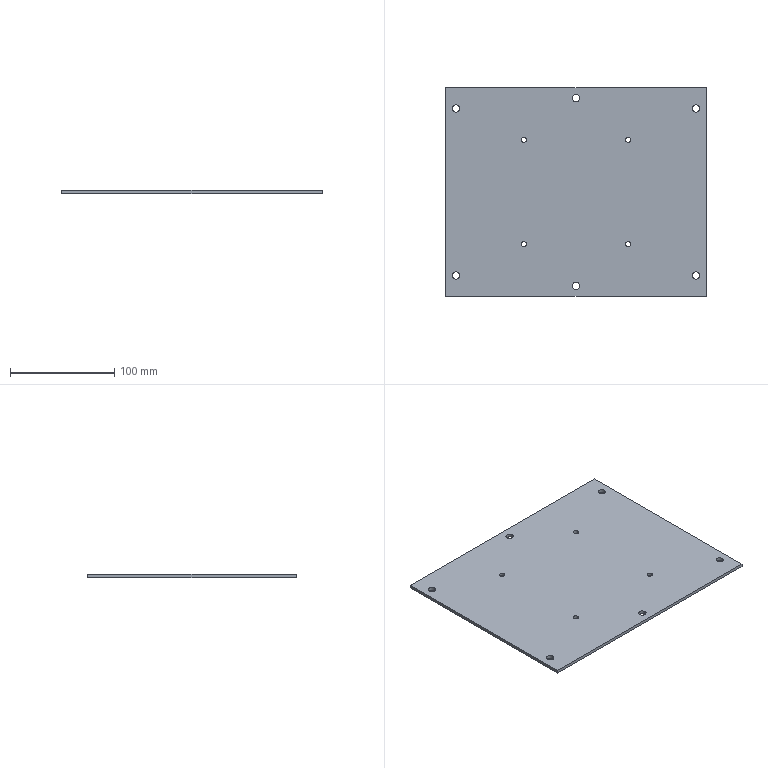Part | SolidWorks | features Cut 2, FlatPattern 1, HoleWzd 1, SMBaseFlange 1, SheetMetal 1 | 1 solid | 26 faces | box 250 x 200 x 3 mm | volume 149072 mm3 | cylinder 20 | plane 6 | commonest cylinder face diameters 7 x12 5 x8
STEP:
#1=CARTESIAN_POINT('',(52.5,50.,0.));
#2=VERTEX_POINT('',#1);
#3=CARTESIAN_POINT('',(47.5,50.,0.));
#4=VERTEX_POINT('',#3);
#5=CARTESIAN_POINT('',(50.,50.,0.));
#6=DIRECTION('',(0.,0.,-1.));
#7=DIRECTION('',(-1.,0.,0.));
#8=AXIS2_PLACEMENT_3D('',#5,#6,#7);
#9=CIRCLE('',#8,2.5);
#10=EDGE_CURVE('',#2,#4,#9,.T.);
#11=ORIENTED_EDGE('',*,*,#10,.F.);
#12=CARTESIAN_POINT('',(52.5,50.,-3.));
#13=VERTEX_POINT('',#12);
#14=CARTESIAN_POINT('',(52.5,50.,-3.));
#15=DIRECTION('',(0.,0.,-1.));
#16=VECTOR('',#15,1000.);
#17=LINE('',#14,#16);
#18=EDGE_CURVE('',#2,#13,#17,.T.);
#19=ORIENTED_EDGE('',*,*,#18,.T.);
#20=CARTESIAN_POINT('',(47.5,50.,-3.));
#21=VERTEX_POINT('',#20);
#22=CARTESIAN_POINT('',(50.,50.,-3.));
#23=DIRECTION('',(0.,0.,-1.));
#24=DIRECTION('',(-1.,0.,0.));
#25=AXIS2_PLACEMENT_3D('',#22,#23,#24);
#26=CIRCLE('',#25,2.5);
#27=EDGE_CURVE('',#13,#21,#26,.T.);
#28=ORIENTED_EDGE('',*,*,#27,.T.);
#29=CARTESIAN_POINT('',(47.5,50.,-3.));
#30=DIRECTION('',(0.,0.,-1.));
#31=VECTOR('',#30,1000.);
#32=LINE('',#29,#31);
#33=EDGE_CURVE('',#4,#21,#32,.T.);
#34=ORIENTED_EDGE('',*,*,#33,.F.);
#35=EDGE_LOOP('',(#11,#19,#28,#34));
#36=FACE_OUTER_BOUND('',#35,.T.);
#37=CARTESIAN_POINT('',(50.,50.,-3.));
#38=DIRECTION('',(0.,0.,-1.));
#39=DIRECTION('',(-1.,0.,0.));
#40=AXIS2_PLACEMENT_3D('',#37,#38,#39);
#41=CYLINDRICAL_SURFACE('',#40,2.5);
#42=ADVANCED_FACE('',(#36),#41,.F.);
#43=CARTESIAN_POINT('',(-47.5,50.,0.));
#44=VERTEX_POINT('',#43);
#45=CARTESIAN_POINT('',(-52.5,50.,0.));
#46=VERTEX_POINT('',#45);
#47=CARTESIAN_POINT('',(-50.,50.,0.));
#48=DIRECTION('',(0.,0.,-1.));
#49=DIRECTION('',(-1.,0.,0.));
#50=AXIS2_PLACEMENT_3D('',#47,#48,#49);
#51=CIRCLE('',#50,2.5);
#52=EDGE_CURVE('',#44,#46,#51,.T.);
#53=ORIENTED_EDGE('',*,*,#52,.F.);
#54=CARTESIAN_POINT('',(-47.5,50.,-3.));
#55=VERTEX_POINT('',#54);
#56=CARTESIAN_POINT('',(-47.5,50.,-3.));
#57=DIRECTION('',(0.,0.,-1.));
#58=VECTOR('',#57,1000.);
#59=LINE('',#56,#58);
#60=EDGE_CURVE('',#44,#55,#59,.T.);
#61=ORIENTED_EDGE('',*,*,#60,.T.);
#62=CARTESIAN_POINT('',(-52.5,50.,-3.));
#63=VERTEX_POINT('',#62);
#64=CARTESIAN_POINT('',(-50.,50.,-3.));
#65=DIRECTION('',(0.,0.,-1.));
#66=DIRECTION('',(-1.,0.,0.));
#67=AXIS2_PLACEMENT_3D('',#64,#65,#66);
#68=CIRCLE('',#67,2.5);
#69=EDGE_CURVE('',#55,#63,#68,.T.);
#70=ORIENTED_EDGE('',*,*,#69,.T.);
#71=CARTESIAN_POINT('',(-52.5,50.,-3.));
#72=DIRECTION('',(0.,0.,-1.));
#73=VECTOR('',#72,1000.);
#74=LINE('',#71,#73);
#75=EDGE_CURVE('',#46,#63,#74,.T.);
#76=ORIENTED_EDGE('',*,*,#75,.F.);
#77=EDGE_LOOP('',(#53,#61,#70,#76));
#78=FACE_OUTER_BOUND('',#77,.T.);
#79=CARTESIAN_POINT('',(-50.,50.,-3.));
#80=DIRECTION('',(0.,0.,-1.));
#81=DIRECTION('',(-1.,0.,0.));
#82=AXIS2_PLACEMENT_3D('',#79,#80,#81);
#83=CYLINDRICAL_SURFACE('',#82,2.5);
#84=ADVANCED_FACE('',(#78),#83,.F.);
#85=CARTESIAN_POINT('',(-47.5,-50.,0.));
#86=VERTEX_POINT('',#85);
#87=CARTESIAN_POINT('',(-52.5,-50.,0.));
#88=VERTEX_POINT('',#87);
#89=CARTESIAN_POINT('',(-50.,-50.,0.));
#90=DIRECTION('',(0.,0.,-1.));
#91=DIRECTION('',(-1.,0.,0.));
#92=AXIS2_PLACEMENT_3D('',#89,#90,#91);
#93=CIRCLE('',#92,2.5);
#94=EDGE_CURVE('',#86,#88,#93,.T.);
#95=ORIENTED_EDGE('',*,*,#94,.F.);
#96=CARTESIAN_POINT('',(-47.5,-50.,-3.));
#97=VERTEX_POINT('',#96);
#98=CARTESIAN_POINT('',(-47.5,-50.,-3.));
#99=DIRECTION('',(0.,0.,-1.));
#100=VECTOR('',#99,1000.);
#101=LINE('',#98,#100);
#102=EDGE_CURVE('',#86,#97,#101,.T.);
#103=ORIENTED_EDGE('',*,*,#102,.T.);
#104=CARTESIAN_POINT('',(-52.5,-50.,-3.));
#105=VERTEX_POINT('',#104);
#106=CARTESIAN_POINT('',(-50.,-50.,-3.));
#107=DIRECTION('',(0.,0.,-1.));
#108=DIRECTION('',(-1.,0.,0.));
#109=AXIS2_PLACEMENT_3D('',#106,#107,#108);
#110=CIRCLE('',#109,2.5);
#111=EDGE_CURVE('',#97,#105,#110,.T.);
#112=ORIENTED_EDGE('',*,*,#111,.T.);
#113=CARTESIAN_POINT('',(-52.5,-50.,-3.));
#114=DIRECTION('',(0.,0.,-1.));
#115=VECTOR('',#114,1000.);
#116=LINE('',#113,#115);
#117=EDGE_CURVE('',#88,#105,#116,.T.);
#118=ORIENTED_EDGE('',*,*,#117,.F.);
#119=EDGE_LOOP('',(#95,#103,#112,#118));
#120=FACE_OUTER_BOUND('',#119,.T.);
#121=CARTESIAN_POINT('',(-50.,-50.,-3.));
#122=DIRECTION('',(0.,0.,-1.));
#123=DIRECTION('',(-1.,0.,0.));
#124=AXIS2_PLACEMENT_3D('',#121,#122,#123);
#125=CYLINDRICAL_SURFACE('',#124,2.5);
#126=ADVANCED_FACE('',(#120),#125,.F.);
#127=CARTESIAN_POINT('',(52.5,-50.,0.));
#128=VERTEX_POINT('',#127);
#129=CARTESIAN_POINT('',(47.5,-50.,0.));
#130=VERTEX_POINT('',#129);
#131=CARTESIAN_POINT('',(50.,-50.,0.));
#132=DIRECTION('',(0.,0.,-1.));
#133=DIRECTION('',(-1.,0.,0.));
#134=AXIS2_PLACEMENT_3D('',#131,#132,#133);
#135=CIRCLE('',#134,2.5);
#136=EDGE_CURVE('',#128,#130,#135,.T.);
#137=ORIENTED_EDGE('',*,*,#136,.F.);
#138=CARTESIAN_POINT('',(52.5,-50.,-3.));
#139=VERTEX_POINT('',#138);
#140=CARTESIAN_POINT('',(52.5,-50.,-3.));
#141=DIRECTION('',(0.,0.,-1.));
#142=VECTOR('',#141,1000.);
#143=LINE('',#140,#142);
#144=EDGE_CURVE('',#128,#139,#143,.T.);
#145=ORIENTED_EDGE('',*,*,#144,.T.);
#146=CARTESIAN_POINT('',(47.5,-50.,-3.));
#147=VERTEX_POINT('',#146);
#148=CARTESIAN_POINT('',(50.,-50.,-3.));
#149=DIRECTION('',(0.,0.,-1.));
#150=DIRECTION('',(-1.,0.,0.));
#151=AXIS2_PLACEMENT_3D('',#148,#149,#150);
#152=CIRCLE('',#151,2.5);
#153=EDGE_CURVE('',#139,#147,#152,.T.);
#154=ORIENTED_EDGE('',*,*,#153,.T.);
#155=CARTESIAN_POINT('',(47.5,-50.,-3.));
#156=DIRECTION('',(0.,0.,-1.));
#157=VECTOR('',#156,1000.);
#158=LINE('',#155,#157);
#159=EDGE_CURVE('',#130,#147,#158,.T.);
#160=ORIENTED_EDGE('',*,*,#159,.F.);
#161=EDGE_LOOP('',(#137,#145,#154,#160));
#162=FACE_OUTER_BOUND('',#161,.T.);
#163=CARTESIAN_POINT('',(50.,-50.,-3.));
#164=DIRECTION('',(0.,0.,-1.));
#165=DIRECTION('',(-1.,0.,0.));
#166=AXIS2_PLACEMENT_3D('',#163,#164,#165);
#167=CYLINDRICAL_SURFACE('',#166,2.5);
#168=ADVANCED_FACE('',(#162),#167,.F.);
#169=CARTESIAN_POINT('',(3.5,-90.,0.));
#170=VERTEX_POINT('',#169);
#171=CARTESIAN_POINT('',(-3.5,-90.,0.));
#172=VERTEX_POINT('',#171);
#173=CARTESIAN_POINT('',(0.,-90.,0.));
#174=DIRECTION('',(0.,0.,-1.));
#175=DIRECTION('',(1.,0.,0.));
#176=AXIS2_PLACEMENT_3D('',#173,#174,#175);
#177=CIRCLE('',#176,3.5);
#178=EDGE_CURVE('',#170,#172,#177,.T.);
#179=ORIENTED_EDGE('',*,*,#178,.F.);
#180=CARTESIAN_POINT('',(3.5,-90.,-3.));
#181=VERTEX_POINT('',#180);
#182=CARTESIAN_POINT('',(3.5,-90.,0.001));
#183=DIRECTION('',(0.,0.,-1.));
#184=VECTOR('',#183,1000.);
#185=LINE('',#182,#184);
#186=EDGE_CURVE('',#170,#181,#185,.T.);
#187=ORIENTED_EDGE('',*,*,#186,.T.);
#188=CARTESIAN_POINT('',(-3.5,-90.,-3.));
#189=VERTEX_POINT('',#188);
#190=CARTESIAN_POINT('',(0.,-90.,-3.));
#191=DIRECTION('',(0.,0.,-1.));
#192=DIRECTION('',(-1.,0.,0.));
#193=AXIS2_PLACEMENT_3D('',#190,#191,#192);
#194=CIRCLE('',#193,3.5);
#195=EDGE_CURVE('',#181,#189,#194,.T.);
#196=ORIENTED_EDGE('',*,*,#195,.T.);
#197=CARTESIAN_POINT('',(-3.5,-90.,0.001));
#198=DIRECTION('',(0.,0.,-1.));
#199=VECTOR('',#198,1000.);
#200=LINE('',#197,#199);
#201=EDGE_CURVE('',#172,#189,#200,.T.);
#202=ORIENTED_EDGE('',*,*,#201,.F.);
#203=EDGE_LOOP('',(#179,#187,#196,#202));
#204=FACE_OUTER_BOUND('',#203,.T.);
#205=CARTESIAN_POINT('',(0.,-90.,0.001));
#206=DIRECTION('',(0.,0.,-1.));
#207=DIRECTION('',(-1.,0.,0.));
#208=AXIS2_PLACEMENT_3D('',#205,#206,#207);
#209=CYLINDRICAL_SURFACE('',#208,3.5);
#210=ADVANCED_FACE('',(#204),#209,.F.);
#211=CARTESIAN_POINT('',(3.5,90.,0.));
#212=VERTEX_POINT('',#211);
#213=CARTESIAN_POINT('',(-3.5,90.,0.));
#214=VERTEX_POINT('',#213);
#215=CARTESIAN_POINT('',(0.,90.,0.));
#216=DIRECTION('',(0.,0.,-1.));
#217=DIRECTION('',(1.,0.,0.));
#218=AXIS2_PLACEMENT_3D('',#215,#216,#217);
#219=CIRCLE('',#218,3.5);
#220=EDGE_CURVE('',#212,#214,#219,.T.);
#221=ORIENTED_EDGE('',*,*,#220,.F.);
#222=CARTESIAN_POINT('',(3.5,90.,-3.));
#223=VERTEX_POINT('',#222);
#224=CARTESIAN_POINT('',(3.5,90.,0.001));
#225=DIRECTION('',(0.,0.,-1.));
#226=VECTOR('',#225,1000.);
#227=LINE('',#224,#226);
#228=EDGE_CURVE('',#212,#223,#227,.T.);
#229=ORIENTED_EDGE('',*,*,#228,.T.);
#230=CARTESIAN_POINT('',(-3.5,90.,-3.));
#231=VERTEX_POINT('',#230);
#232=CARTESIAN_POINT('',(0.,90.,-3.));
#233=DIRECTION('',(0.,0.,-1.));
#234=DIRECTION('',(-1.,0.,0.));
#235=AXIS2_PLACEMENT_3D('',#232,#233,#234);
#236=CIRCLE('',#235,3.5);
#237=EDGE_CURVE('',#223,#231,#236,.T.);
#238=ORIENTED_EDGE('',*,*,#237,.T.);
#239=CARTESIAN_POINT('',(-3.5,90.,0.001));
#240=DIRECTION('',(0.,0.,-1.));
#241=VECTOR('',#240,1000.);
#242=LINE('',#239,#241);
#243=EDGE_CURVE('',#214,#231,#242,.T.);
#244=ORIENTED_EDGE('',*,*,#243,.F.);
#245=EDGE_LOOP('',(#221,#229,#238,#244));
#246=FACE_OUTER_BOUND('',#245,.T.);
#247=CARTESIAN_POINT('',(0.,90.,0.001));
#248=DIRECTION('',(0.,0.,-1.));
#249=DIRECTION('',(-1.,0.,0.));
#250=AXIS2_PLACEMENT_3D('',#247,#248,#249);
#251=CYLINDRICAL_SURFACE('',#250,3.5);
#252=ADVANCED_FACE('',(#246),#251,.F.);
#253=CARTESIAN_POINT('',(118.5,-80.,0.));
#254=VERTEX_POINT('',#253);
#255=CARTESIAN_POINT('',(111.5,-80.,0.));
#256=VERTEX_POINT('',#255);
#257=CARTESIAN_POINT('',(115.,-80.,0.));
#258=DIRECTION('',(0.,0.,-1.));
#259=DIRECTION('',(1.,0.,0.));
#260=AXIS2_PLACEMENT_3D('',#257,#258,#259);
#261=CIRCLE('',#260,3.5);
#262=EDGE_CURVE('',#254,#256,#261,.T.);
#263=ORIENTED_EDGE('',*,*,#262,.F.);
#264=CARTESIAN_POINT('',(118.5,-80.,-3.));
#265=VERTEX_POINT('',#264);
#266=CARTESIAN_POINT('',(118.5,-80.,0.001));
#267=DIRECTION('',(0.,0.,-1.));
#268=VECTOR('',#267,1000.);
#269=LINE('',#266,#268);
#270=EDGE_CURVE('',#254,#265,#269,.T.);
#271=ORIENTED_EDGE('',*,*,#270,.T.);
#272=CARTESIAN_POINT('',(111.5,-80.,-3.));
#273=VERTEX_POINT('',#272);
#274=CARTESIAN_POINT('',(115.,-80.,-3.));
#275=DIRECTION('',(0.,0.,-1.));
#276=DIRECTION('',(-1.,0.,0.));
#277=AXIS2_PLACEMENT_3D('',#274,#275,#276);
#278=CIRCLE('',#277,3.5);
#279=EDGE_CURVE('',#265,#273,#278,.T.);
#280=ORIENTED_EDGE('',*,*,#279,.T.);
#281=CARTESIAN_POINT('',(111.5,-80.,0.001));
#282=DIRECTION('',(0.,0.,-1.));
#283=VECTOR('',#282,1000.);
#284=LINE('',#281,#283);
#285=EDGE_CURVE('',#256,#273,#284,.T.);
#286=ORIENTED_EDGE('',*,*,#285,.F.);
#287=EDGE_LOOP('',(#263,#271,#280,#286));
#288=FACE_OUTER_BOUND('',#287,.T.);
#289=CARTESIAN_POINT('',(115.,-80.,0.001));
#290=DIRECTION('',(0.,0.,-1.));
#291=DIRECTION('',(-1.,0.,0.));
#292=AXIS2_PLACEMENT_3D('',#289,#290,#291);
#293=CYLINDRICAL_SURFACE('',#292,3.5);
#294=ADVANCED_FACE('',(#288),#293,.F.);
#295=CARTESIAN_POINT('',(-111.5,-80.,0.));
#296=VERTEX_POINT('',#295);
#297=CARTESIAN_POINT('',(-118.5,-80.,0.));
#298=VERTEX_POINT('',#297);
#299=CARTESIAN_POINT('',(-115.,-80.,0.));
#300=DIRECTION('',(0.,0.,-1.));
#301=DIRECTION('',(1.,0.,0.));
#302=AXIS2_PLACEMENT_3D('',#299,#300,#301);
#303=CIRCLE('',#302,3.5);
#304=EDGE_CURVE('',#296,#298,#303,.T.);
#305=ORIENTED_EDGE('',*,*,#304,.F.);
#306=CARTESIAN_POINT('',(-111.5,-80.,-3.));
#307=VERTEX_POINT('',#306);
#308=CARTESIAN_POINT('',(-111.5,-80.,0.001));
#309=DIRECTION('',(0.,0.,-1.));
#310=VECTOR('',#309,1000.);
#311=LINE('',#308,#310);
#312=EDGE_CURVE('',#296,#307,#311,.T.);
#313=ORIENTED_EDGE('',*,*,#312,.T.);
#314=CARTESIAN_POINT('',(-118.5,-80.,-3.));
#315=VERTEX_POINT('',#314);
#316=CARTESIAN_POINT('',(-115.,-80.,-3.));
#317=DIRECTION('',(0.,0.,-1.));
#318=DIRECTION('',(-1.,0.,0.));
#319=AXIS2_PLACEMENT_3D('',#316,#317,#318);
#320=CIRCLE('',#319,3.5);
#321=EDGE_CURVE('',#307,#315,#320,.T.);
#322=ORIENTED_EDGE('',*,*,#321,.T.);
#323=CARTESIAN_POINT('',(-118.5,-80.,0.001));
#324=DIRECTION('',(0.,0.,-1.));
#325=VECTOR('',#324,1000.);
#326=LINE('',#323,#325);
#327=EDGE_CURVE('',#298,#315,#326,.T.);
#328=ORIENTED_EDGE('',*,*,#327,.F.);
#329=EDGE_LOOP('',(#305,#313,#322,#328));
#330=FACE_OUTER_BOUND('',#329,.T.);
#331=CARTESIAN_POINT('',(-115.,-80.,0.001));
#332=DIRECTION('',(0.,0.,-1.));
#333=DIRECTION('',(-1.,0.,0.));
#334=AXIS2_PLACEMENT_3D('',#331,#332,#333);
#335=CYLINDRICAL_SURFACE('',#334,3.5);
#336=ADVANCED_FACE('',(#330),#335,.F.);
#337=CARTESIAN_POINT('',(-111.5,80.,0.));
#338=VERTEX_POINT('',#337);
#339=CARTESIAN_POINT('',(-118.5,80.,0.));
#340=VERTEX_POINT('',#339);
#341=CARTESIAN_POINT('',(-115.,80.,0.));
#342=DIRECTION('',(0.,0.,-1.));
#343=DIRECTION('',(1.,0.,0.));
#344=AXIS2_PLACEMENT_3D('',#341,#342,#343);
#345=CIRCLE('',#344,3.5);
#346=EDGE_CURVE('',#338,#340,#345,.T.);
#347=ORIENTED_EDGE('',*,*,#346,.F.);
#348=CARTESIAN_POINT('',(-111.5,80.,-3.));
#349=VERTEX_POINT('',#348);
#350=CARTESIAN_POINT('',(-111.5,80.,0.001));
#351=DIRECTION('',(0.,0.,-1.));
#352=VECTOR('',#351,1000.);
#353=LINE('',#350,#352);
#354=EDGE_CURVE('',#338,#349,#353,.T.);
#355=ORIENTED_EDGE('',*,*,#354,.T.);
#356=CARTESIAN_POINT('',(-118.5,80.,-3.));
#357=VERTEX_POINT('',#356);
#358=CARTESIAN_POINT('',(-115.,80.,-3.));
#359=DIRECTION('',(0.,0.,-1.));
#360=DIRECTION('',(-1.,0.,0.));
#361=AXIS2_PLACEMENT_3D('',#358,#359,#360);
#362=CIRCLE('',#361,3.5);
#363=EDGE_CURVE('',#349,#357,#362,.T.);
#364=ORIENTED_EDGE('',*,*,#363,.T.);
#365=CARTESIAN_POINT('',(-118.5,80.,0.001));
#366=DIRECTION('',(0.,0.,-1.));
#367=VECTOR('',#366,1000.);
#368=LINE('',#365,#367);
#369=EDGE_CURVE('',#340,#357,#368,.T.);
#370=ORIENTED_EDGE('',*,*,#369,.F.);
#371=EDGE_LOOP('',(#347,#355,#364,#370));
#372=FACE_OUTER_BOUND('',#371,.T.);
#373=CARTESIAN_POINT('',(-115.,80.,0.001));
#374=DIRECTION('',(0.,0.,-1.));
#375=DIRECTION('',(-1.,0.,0.));
#376=AXIS2_PLACEMENT_3D('',#373,#374,#375);
#377=CYLINDRICAL_SURFACE('',#376,3.5);
#378=ADVANCED_FACE('',(#372),#377,.F.);
#379=CARTESIAN_POINT('',(118.5,80.,0.));
#380=VERTEX_POINT('',#379);
#381=CARTESIAN_POINT('',(111.5,80.,0.));
#382=VERTEX_POINT('',#381);
#383=CARTESIAN_POINT('',(115.,80.,0.));
#384=DIRECTION('',(0.,0.,-1.));
#385=DIRECTION('',(1.,0.,0.));
#386=AXIS2_PLACEMENT_3D('',#383,#384,#385);
#387=CIRCLE('',#386,3.5);
#388=EDGE_CURVE('',#380,#382,#387,.T.);
#389=ORIENTED_EDGE('',*,*,#388,.F.);
#390=CARTESIAN_POINT('',(118.5,80.,-3.));
#391=VERTEX_POINT('',#390);
#392=CARTESIAN_POINT('',(118.5,80.,0.001));
#393=DIRECTION('',(0.,0.,-1.));
#394=VECTOR('',#393,1000.);
#395=LINE('',#392,#394);
#396=EDGE_CURVE('',#380,#391,#395,.T.);
#397=ORIENTED_EDGE('',*,*,#396,.T.);
#398=CARTESIAN_POINT('',(111.5,80.,-3.));
#399=VERTEX_POINT('',#398);
#400=CARTESIAN_POINT('',(115.,80.,-3.));
#401=DIRECTION('',(0.,0.,-1.));
#402=DIRECTION('',(-1.,0.,0.));
#403=AXIS2_PLACEMENT_3D('',#400,#401,#402);
#404=CIRCLE('',#403,3.5);
#405=EDGE_CURVE('',#391,#399,#404,.T.);
#406=ORIENTED_EDGE('',*,*,#405,.T.);
#407=CARTESIAN_POINT('',(111.5,80.,0.001));
#408=DIRECTION('',(0.,0.,-1.));
#409=VECTOR('',#408,1000.);
#410=LINE('',#407,#409);
#411=EDGE_CURVE('',#382,#399,#410,.T.);
#412=ORIENTED_EDGE('',*,*,#411,.F.);
#413=EDGE_LOOP('',(#389,#397,#406,#412));
#414=FACE_OUTER_BOUND('',#413,.T.);
#415=CARTESIAN_POINT('',(115.,80.,0.001));
#416=DIRECTION('',(0.,0.,-1.));
#417=DIRECTION('',(-1.,0.,0.));
#418=AXIS2_PLACEMENT_3D('',#415,#416,#417);
#419=CYLINDRICAL_SURFACE('',#418,3.5);
#420=ADVANCED_FACE('',(#414),#419,.F.);
#421=CARTESIAN_POINT('',(125.,-100.,0.));
#422=VERTEX_POINT('',#421);
#423=CARTESIAN_POINT('',(125.,100.,0.));
#424=VERTEX_POINT('',#423);
#425=CARTESIAN_POINT('',(125.,100.,0.));
#426=DIRECTION('',(0.,1.,0.));
#427=VECTOR('',#426,1000.);
#428=LINE('',#425,#427);
#429=EDGE_CURVE('',#422,#424,#428,.T.);
#430=ORIENTED_EDGE('',*,*,#429,.F.);
#431=CARTESIAN_POINT('',(125.,-100.,-3.));
#432=VERTEX_POINT('',#431);
#433=CARTESIAN_POINT('',(125.,-100.,-3.));
#434=DIRECTION('',(0.,0.,1.));
#435=VECTOR('',#434,1000.);
#436=LINE('',#433,#435);
#437=EDGE_CURVE('',#432,#422,#436,.T.);
#438=ORIENTED_EDGE('',*,*,#437,.F.);
#439=CARTESIAN_POINT('',(125.,100.,-3.));
#440=VERTEX_POINT('',#439);
#441=CARTESIAN_POINT('',(125.,100.,-3.));
#442=DIRECTION('',(0.,1.,0.));
#443=VECTOR('',#442,1000.);
#444=LINE('',#441,#443);
#445=EDGE_CURVE('',#432,#440,#444,.T.);
#446=ORIENTED_EDGE('',*,*,#445,.T.);
#447=CARTESIAN_POINT('',(125.,100.,-3.));
#448=DIRECTION('',(0.,0.,1.));
#449=VECTOR('',#448,1000.);
#450=LINE('',#447,#449);
#451=EDGE_CURVE('',#440,#424,#450,.T.);
#452=ORIENTED_EDGE('',*,*,#451,.T.);
#453=EDGE_LOOP('',(#430,#438,#446,#452));
#454=FACE_OUTER_BOUND('',#453,.T.);
#455=CARTESIAN_POINT('',(125.,100.,-3.));
#456=DIRECTION('',(1.,0.,0.));
#457=DIRECTION('',(0.,1.,0.));
#458=AXIS2_PLACEMENT_3D('',#455,#456,#457);
#459=PLANE('',#458);
#460=ADVANCED_FACE('',(#454),#459,.T.);
#461=CARTESIAN_POINT('',(-125.,-100.,0.));
#462=VERTEX_POINT('',#461);
#463=CARTESIAN_POINT('',(-125.,-100.,0.));
#464=DIRECTION('',(1.,0.,0.));
#465=VECTOR('',#464,1000.);
#466=LINE('',#463,#465);
#467=EDGE_CURVE('',#462,#422,#466,.T.);
#468=ORIENTED_EDGE('',*,*,#467,.F.);
#469=CARTESIAN_POINT('',(-125.,-100.,-3.));
#470=VERTEX_POINT('',#469);
#471=CARTESIAN_POINT('',(-125.,-100.,-3.));
#472=DIRECTION('',(0.,0.,1.));
#473=VECTOR('',#472,1000.);
#474=LINE('',#471,#473);
#475=EDGE_CURVE('',#470,#462,#474,.T.);
#476=ORIENTED_EDGE('',*,*,#475,.F.);
#477=CARTESIAN_POINT('',(-125.,-100.,-3.));
#478=DIRECTION('',(1.,0.,0.));
#479=VECTOR('',#478,1000.);
#480=LINE('',#477,#479);
#481=EDGE_CURVE('',#470,#432,#480,.T.);
#482=ORIENTED_EDGE('',*,*,#481,.T.);
#483=ORIENTED_EDGE('',*,*,#437,.T.);
#484=EDGE_LOOP('',(#468,#476,#482,#483));
#485=FACE_OUTER_BOUND('',#484,.T.);
#486=CARTESIAN_POINT('',(-125.,-100.,-3.));
#487=DIRECTION('',(0.,-1.,0.));
#488=DIRECTION('',(0.,0.,-1.));
#489=AXIS2_PLACEMENT_3D('',#486,#487,#488);
#490=PLANE('',#489);
#491=ADVANCED_FACE('',(#485),#490,.T.);
#492=CARTESIAN_POINT('',(-125.,100.,0.));
#493=VERTEX_POINT('',#492);
#494=CARTESIAN_POINT('',(-125.,100.,0.));
#495=DIRECTION('',(0.,-1.,0.));
#496=VECTOR('',#495,1000.);
#497=LINE('',#494,#496);
#498=EDGE_CURVE('',#493,#462,#497,.T.);
#499=ORIENTED_EDGE('',*,*,#498,.F.);
#500=CARTESIAN_POINT('',(-125.,100.,-3.));
#501=VERTEX_POINT('',#500);
#502=CARTESIAN_POINT('',(-125.,100.,-3.));
#503=DIRECTION('',(0.,0.,1.));
#504=VECTOR('',#503,1000.);
#505=LINE('',#502,#504);
#506=EDGE_CURVE('',#501,#493,#505,.T.);
#507=ORIENTED_EDGE('',*,*,#506,.F.);
#508=CARTESIAN_POINT('',(-125.,100.,-3.));
#509=DIRECTION('',(0.,-1.,0.));
#510=VECTOR('',#509,1000.);
#511=LINE('',#508,#510);
#512=EDGE_CURVE('',#501,#470,#511,.T.);
#513=ORIENTED_EDGE('',*,*,#512,.T.);
#514=ORIENTED_EDGE('',*,*,#475,.T.);
#515=EDGE_LOOP('',(#499,#507,#513,#514));
#516=FACE_OUTER_BOUND('',#515,.T.);
#517=CARTESIAN_POINT('',(-125.,100.,-3.));
#518=DIRECTION('',(-1.,0.,0.));
#519=DIRECTION('',(0.,-1.,0.));
#520=AXIS2_PLACEMENT_3D('',#517,#518,#519);
#521=PLANE('',#520);
#522=ADVANCED_FACE('',(#516),#521,.T.);
#523=CARTESIAN_POINT('',(-125.,100.,0.));
#524=DIRECTION('',(-1.,0.,0.));
#525=VECTOR('',#524,1000.);
#526=LINE('',#523,#525);
#527=EDGE_CURVE('',#424,#493,#526,.T.);
#528=ORIENTED_EDGE('',*,*,#527,.F.);
#529=ORIENTED_EDGE('',*,*,#451,.F.);
#530=CARTESIAN_POINT('',(-125.,100.,-3.));
#531=DIRECTION('',(-1.,0.,0.));
#532=VECTOR('',#531,1000.);
#533=LINE('',#530,#532);
#534=EDGE_CURVE('',#440,#501,#533,.T.);
#535=ORIENTED_EDGE('',*,*,#534,.T.);
#536=ORIENTED_EDGE('',*,*,#506,.T.);
#537=EDGE_LOOP('',(#528,#529,#535,#536));
#538=FACE_OUTER_BOUND('',#537,.T.);
#539=CARTESIAN_POINT('',(-125.,100.,-3.));
#540=DIRECTION('',(0.,1.,0.));
#541=DIRECTION('',(-1.,0.,0.));
#542=AXIS2_PLACEMENT_3D('',#539,#540,#541);
#543=PLANE('',#542);
#544=ADVANCED_FACE('',(#538),#543,.T.);
#545=CARTESIAN_POINT('',(50.,50.,-3.));
#546=DIRECTION('',(0.,0.,-1.));
#547=DIRECTION('',(-1.,0.,0.));
#548=AXIS2_PLACEMENT_3D('',#545,#546,#547);
#549=CIRCLE('',#548,2.5);
#550=EDGE_CURVE('',#21,#13,#549,.T.);
#551=ORIENTED_EDGE('',*,*,#550,.F.);
#552=ORIENTED_EDGE('',*,*,#27,.F.);
#553=EDGE_LOOP('',(#551,#552));
#554=FACE_BOUND('',#553,.T.);
#555=CARTESIAN_POINT('',(-50.,50.,-3.));
#556=DIRECTION('',(0.,0.,-1.));
#557=DIRECTION('',(-1.,0.,0.));
#558=AXIS2_PLACEMENT_3D('',#555,#556,#557);
#559=CIRCLE('',#558,2.5);
#560=EDGE_CURVE('',#63,#55,#559,.T.);
#561=ORIENTED_EDGE('',*,*,#560,.F.);
#562=ORIENTED_EDGE('',*,*,#69,.F.);
#563=EDGE_LOOP('',(#561,#562));
#564=FACE_BOUND('',#563,.T.);
#565=CARTESIAN_POINT('',(-50.,-50.,-3.));
#566=DIRECTION('',(0.,0.,-1.));
#567=DIRECTION('',(-1.,0.,0.));
#568=AXIS2_PLACEMENT_3D('',#565,#566,#567);
#569=CIRCLE('',#568,2.5);
#570=EDGE_CURVE('',#105,#97,#569,.T.);
#571=ORIENTED_EDGE('',*,*,#570,.F.);
#572=ORIENTED_EDGE('',*,*,#111,.F.);
#573=EDGE_LOOP('',(#571,#572));
#574=FACE_BOUND('',#573,.T.);
#575=CARTESIAN_POINT('',(50.,-50.,-3.));
#576=DIRECTION('',(0.,0.,-1.));
#577=DIRECTION('',(-1.,0.,0.));
#578=AXIS2_PLACEMENT_3D('',#575,#576,#577);
#579=CIRCLE('',#578,2.5);
#580=EDGE_CURVE('',#147,#139,#579,.T.);
#581=ORIENTED_EDGE('',*,*,#580,.F.);
#582=ORIENTED_EDGE('',*,*,#153,.F.);
#583=EDGE_LOOP('',(#581,#582));
#584=FACE_BOUND('',#583,.T.);
#585=CARTESIAN_POINT('',(0.,-90.,-3.));
#586=DIRECTION('',(0.,0.,-1.));
#587=DIRECTION('',(-1.,0.,0.));
#588=AXIS2_PLACEMENT_3D('',#585,#586,#587);
#589=CIRCLE('',#588,3.5);
#590=EDGE_CURVE('',#189,#181,#589,.T.);
#591=ORIENTED_EDGE('',*,*,#590,.F.);
#592=ORIENTED_EDGE('',*,*,#195,.F.);
#593=EDGE_LOOP('',(#591,#592));
#594=FACE_BOUND('',#593,.T.);
#595=CARTESIAN_POINT('',(0.,90.,-3.));
#596=DIRECTION('',(0.,0.,-1.));
#597=DIRECTION('',(-1.,0.,0.));
#598=AXIS2_PLACEMENT_3D('',#595,#596,#597);
#599=CIRCLE('',#598,3.5);
#600=EDGE_CURVE('',#231,#223,#599,.T.);
#601=ORIENTED_EDGE('',*,*,#600,.F.);
#602=ORIENTED_EDGE('',*,*,#237,.F.);
#603=EDGE_LOOP('',(#601,#602));
#604=FACE_BOUND('',#603,.T.);
#605=CARTESIAN_POINT('',(115.,-80.,-3.));
#606=DIRECTION('',(0.,0.,-1.));
#607=DIRECTION('',(-1.,0.,0.));
#608=AXIS2_PLACEMENT_3D('',#605,#606,#607);
#609=CIRCLE('',#608,3.5);
#610=EDGE_CURVE('',#273,#265,#609,.T.);
#611=ORIENTED_EDGE('',*,*,#610,.F.);
#612=ORIENTED_EDGE('',*,*,#279,.F.);
#613=EDGE_LOOP('',(#611,#612));
#614=FACE_BOUND('',#613,.T.);
#615=CARTESIAN_POINT('',(-115.,-80.,-3.));
#616=DIRECTION('',(0.,0.,-1.));
#617=DIRECTION('',(-1.,0.,0.));
#618=AXIS2_PLACEMENT_3D('',#615,#616,#617);
#619=CIRCLE('',#618,3.5);
#620=EDGE_CURVE('',#315,#307,#619,.T.);
#621=ORIENTED_EDGE('',*,*,#620,.F.);
#622=ORIENTED_EDGE('',*,*,#321,.F.);
#623=EDGE_LOOP('',(#621,#622));
#624=FACE_BOUND('',#623,.T.);
#625=CARTESIAN_POINT('',(-115.,80.,-3.));
#626=DIRECTION('',(0.,0.,-1.));
#627=DIRECTION('',(-1.,0.,0.));
#628=AXIS2_PLACEMENT_3D('',#625,#626,#627);
#629=CIRCLE('',#628,3.5);
#630=EDGE_CURVE('',#357,#349,#629,.T.);
#631=ORIENTED_EDGE('',*,*,#630,.F.);
#632=ORIENTED_EDGE('',*,*,#363,.F.);
#633=EDGE_LOOP('',(#631,#632));
#634=FACE_BOUND('',#633,.T.);
#635=CARTESIAN_POINT('',(115.,80.,-3.));
#636=DIRECTION('',(0.,0.,-1.));
#637=DIRECTION('',(-1.,0.,0.));
#638=AXIS2_PLACEMENT_3D('',#635,#636,#637);
#639=CIRCLE('',#638,3.5);
#640=EDGE_CURVE('',#399,#391,#639,.T.);
#641=ORIENTED_EDGE('',*,*,#640,.F.);
#642=ORIENTED_EDGE('',*,*,#405,.F.);
#643=EDGE_LOOP('',(#641,#642));
#644=FACE_BOUND('',#643,.T.);
#645=ORIENTED_EDGE('',*,*,#445,.F.);
#646=ORIENTED_EDGE('',*,*,#481,.F.);
#647=ORIENTED_EDGE('',*,*,#512,.F.);
#648=ORIENTED_EDGE('',*,*,#534,.F.);
#649=EDGE_LOOP('',(#645,#646,#647,#648));
#650=FACE_OUTER_BOUND('',#649,.T.);
#651=CARTESIAN_POINT('',(0.,0.,-3.));
#652=DIRECTION('',(0.,0.,1.));
#653=DIRECTION('',(1.,0.,0.));
#654=AXIS2_PLACEMENT_3D('',#651,#652,#653);
#655=PLANE('',#654);
#656=ADVANCED_FACE('',(#554,#564,#574,#584,#594,#604,#614,#624,#634,#644,#650),#655,.F.);
#657=CARTESIAN_POINT('',(50.,50.,0.));
#658=DIRECTION('',(0.,0.,-1.));
#659=DIRECTION('',(-1.,0.,0.));
#660=AXIS2_PLACEMENT_3D('',#657,#658,#659);
#661=CIRCLE('',#660,2.5);
#662=EDGE_CURVE('',#4,#2,#661,.T.);
#663=ORIENTED_EDGE('',*,*,#662,.T.);
#664=ORIENTED_EDGE('',*,*,#10,.T.);
#665=EDGE_LOOP('',(#663,#664));
#666=FACE_BOUND('',#665,.T.);
#667=CARTESIAN_POINT('',(-50.,50.,0.));
#668=DIRECTION('',(0.,0.,-1.));
#669=DIRECTION('',(-1.,0.,0.));
#670=AXIS2_PLACEMENT_3D('',#667,#668,#669);
#671=CIRCLE('',#670,2.5);
#672=EDGE_CURVE('',#46,#44,#671,.T.);
#673=ORIENTED_EDGE('',*,*,#672,.T.);
#674=ORIENTED_EDGE('',*,*,#52,.T.);
#675=EDGE_LOOP('',(#673,#674));
#676=FACE_BOUND('',#675,.T.);
#677=CARTESIAN_POINT('',(-50.,-50.,0.));
#678=DIRECTION('',(0.,0.,-1.));
#679=DIRECTION('',(-1.,0.,0.));
#680=AXIS2_PLACEMENT_3D('',#677,#678,#679);
#681=CIRCLE('',#680,2.5);
#682=EDGE_CURVE('',#88,#86,#681,.T.);
#683=ORIENTED_EDGE('',*,*,#682,.T.);
#684=ORIENTED_EDGE('',*,*,#94,.T.);
#685=EDGE_LOOP('',(#683,#684));
#686=FACE_BOUND('',#685,.T.);
#687=CARTESIAN_POINT('',(50.,-50.,0.));
#688=DIRECTION('',(0.,0.,-1.));
#689=DIRECTION('',(-1.,0.,0.));
#690=AXIS2_PLACEMENT_3D('',#687,#688,#689);
#691=CIRCLE('',#690,2.5);
#692=EDGE_CURVE('',#130,#128,#691,.T.);
#693=ORIENTED_EDGE('',*,*,#692,.T.);
#694=ORIENTED_EDGE('',*,*,#136,.T.);
#695=EDGE_LOOP('',(#693,#694));
#696=FACE_BOUND('',#695,.T.);
#697=CARTESIAN_POINT('',(0.,-90.,0.));
#698=DIRECTION('',(0.,0.,-1.));
#699=DIRECTION('',(1.,0.,0.));
#700=AXIS2_PLACEMENT_3D('',#697,#698,#699);
#701=CIRCLE('',#700,3.5);
#702=EDGE_CURVE('',#172,#170,#701,.T.);
#703=ORIENTED_EDGE('',*,*,#702,.T.);
#704=ORIENTED_EDGE('',*,*,#178,.T.);
#705=EDGE_LOOP('',(#703,#704));
#706=FACE_BOUND('',#705,.T.);
#707=CARTESIAN_POINT('',(0.,90.,0.));
#708=DIRECTION('',(0.,0.,-1.));
#709=DIRECTION('',(1.,0.,0.));
#710=AXIS2_PLACEMENT_3D('',#707,#708,#709);
#711=CIRCLE('',#710,3.5);
#712=EDGE_CURVE('',#214,#212,#711,.T.);
#713=ORIENTED_EDGE('',*,*,#712,.T.);
#714=ORIENTED_EDGE('',*,*,#220,.T.);
#715=EDGE_LOOP('',(#713,#714));
#716=FACE_BOUND('',#715,.T.);
#717=CARTESIAN_POINT('',(115.,-80.,0.));
#718=DIRECTION('',(0.,0.,-1.));
#719=DIRECTION('',(1.,0.,0.));
#720=AXIS2_PLACEMENT_3D('',#717,#718,#719);
#721=CIRCLE('',#720,3.5);
#722=EDGE_CURVE('',#256,#254,#721,.T.);
#723=ORIENTED_EDGE('',*,*,#722,.T.);
#724=ORIENTED_EDGE('',*,*,#262,.T.);
#725=EDGE_LOOP('',(#723,#724));
#726=FACE_BOUND('',#725,.T.);
#727=CARTESIAN_POINT('',(-115.,-80.,0.));
#728=DIRECTION('',(0.,0.,-1.));
#729=DIRECTION('',(1.,0.,0.));
#730=AXIS2_PLACEMENT_3D('',#727,#728,#729);
#731=CIRCLE('',#730,3.5);
#732=EDGE_CURVE('',#298,#296,#731,.T.);
#733=ORIENTED_EDGE('',*,*,#732,.T.);
#734=ORIENTED_EDGE('',*,*,#304,.T.);
#735=EDGE_LOOP('',(#733,#734));
#736=FACE_BOUND('',#735,.T.);
#737=CARTESIAN_POINT('',(-115.,80.,0.));
#738=DIRECTION('',(0.,0.,-1.));
#739=DIRECTION('',(1.,0.,0.));
#740=AXIS2_PLACEMENT_3D('',#737,#738,#739);
#741=CIRCLE('',#740,3.5);
#742=EDGE_CURVE('',#340,#338,#741,.T.);
#743=ORIENTED_EDGE('',*,*,#742,.T.);
#744=ORIENTED_EDGE('',*,*,#346,.T.);
#745=EDGE_LOOP('',(#743,#744));
#746=FACE_BOUND('',#745,.T.);
#747=CARTESIAN_POINT('',(115.,80.,0.));
#748=DIRECTION('',(0.,0.,-1.));
#749=DIRECTION('',(1.,0.,0.));
#750=AXIS2_PLACEMENT_3D('',#747,#748,#749);
#751=CIRCLE('',#750,3.5);
#752=EDGE_CURVE('',#382,#380,#751,.T.);
#753=ORIENTED_EDGE('',*,*,#752,.T.);
#754=ORIENTED_EDGE('',*,*,#388,.T.);
#755=EDGE_LOOP('',(#753,#754));
#756=FACE_BOUND('',#755,.T.);
#757=ORIENTED_EDGE('',*,*,#429,.T.);
#758=ORIENTED_EDGE('',*,*,#527,.T.);
#759=ORIENTED_EDGE('',*,*,#498,.T.);
#760=ORIENTED_EDGE('',*,*,#467,.T.);
#761=EDGE_LOOP('',(#757,#758,#759,#760));
#762=FACE_OUTER_BOUND('',#761,.T.);
#763=CARTESIAN_POINT('',(0.,0.,0.));
#764=DIRECTION('',(0.,0.,1.));
#765=DIRECTION('',(1.,0.,0.));
#766=AXIS2_PLACEMENT_3D('',#763,#764,#765);
#767=PLANE('',#766);
#768=ADVANCED_FACE('',(#666,#676,#686,#696,#706,#716,#726,#736,#746,#756,#762),#767,.T.);
#769=ORIENTED_EDGE('',*,*,#396,.F.);
#770=ORIENTED_EDGE('',*,*,#752,.F.);
#771=ORIENTED_EDGE('',*,*,#411,.T.);
#772=ORIENTED_EDGE('',*,*,#640,.T.);
#773=EDGE_LOOP('',(#769,#770,#771,#772));
#774=FACE_OUTER_BOUND('',#773,.T.);
#775=CARTESIAN_POINT('',(115.,80.,0.001));
#776=DIRECTION('',(0.,0.,-1.));
#777=DIRECTION('',(-1.,0.,0.));
#778=AXIS2_PLACEMENT_3D('',#775,#776,#777);
#779=CYLINDRICAL_SURFACE('',#778,3.5);
#780=ADVANCED_FACE('',(#774),#779,.F.);
#781=ORIENTED_EDGE('',*,*,#354,.F.);
#782=ORIENTED_EDGE('',*,*,#742,.F.);
#783=ORIENTED_EDGE('',*,*,#369,.T.);
#784=ORIENTED_EDGE('',*,*,#630,.T.);
#785=EDGE_LOOP('',(#781,#782,#783,#784));
#786=FACE_OUTER_BOUND('',#785,.T.);
#787=CARTESIAN_POINT('',(-115.,80.,0.001));
#788=DIRECTION('',(0.,0.,-1.));
#789=DIRECTION('',(-1.,0.,0.));
#790=AXIS2_PLACEMENT_3D('',#787,#788,#789);
#791=CYLINDRICAL_SURFACE('',#790,3.5);
#792=ADVANCED_FACE('',(#786),#791,.F.);
#793=ORIENTED_EDGE('',*,*,#312,.F.);
#794=ORIENTED_EDGE('',*,*,#732,.F.);
#795=ORIENTED_EDGE('',*,*,#327,.T.);
#796=ORIENTED_EDGE('',*,*,#620,.T.);
#797=EDGE_LOOP('',(#793,#794,#795,#796));
#798=FACE_OUTER_BOUND('',#797,.T.);
#799=CARTESIAN_POINT('',(-115.,-80.,0.001));
#800=DIRECTION('',(0.,0.,-1.));
#801=DIRECTION('',(-1.,0.,0.));
#802=AXIS2_PLACEMENT_3D('',#799,#800,#801);
#803=CYLINDRICAL_SURFACE('',#802,3.5);
#804=ADVANCED_FACE('',(#798),#803,.F.);
#805=ORIENTED_EDGE('',*,*,#270,.F.);
#806=ORIENTED_EDGE('',*,*,#722,.F.);
#807=ORIENTED_EDGE('',*,*,#285,.T.);
#808=ORIENTED_EDGE('',*,*,#610,.T.);
#809=EDGE_LOOP('',(#805,#806,#807,#808));
#810=FACE_OUTER_BOUND('',#809,.T.);
#811=CARTESIAN_POINT('',(115.,-80.,0.001));
#812=DIRECTION('',(0.,0.,-1.));
#813=DIRECTION('',(-1.,0.,0.));
#814=AXIS2_PLACEMENT_3D('',#811,#812,#813);
#815=CYLINDRICAL_SURFACE('',#814,3.5);
#816=ADVANCED_FACE('',(#810),#815,.F.);
#817=ORIENTED_EDGE('',*,*,#228,.F.);
#818=ORIENTED_EDGE('',*,*,#712,.F.);
#819=ORIENTED_EDGE('',*,*,#243,.T.);
#820=ORIENTED_EDGE('',*,*,#600,.T.);
#821=EDGE_LOOP('',(#817,#818,#819,#820));
#822=FACE_OUTER_BOUND('',#821,.T.);
#823=CARTESIAN_POINT('',(0.,90.,0.001));
#824=DIRECTION('',(0.,0.,-1.));
#825=DIRECTION('',(-1.,0.,0.));
#826=AXIS2_PLACEMENT_3D('',#823,#824,#825);
#827=CYLINDRICAL_SURFACE('',#826,3.5);
#828=ADVANCED_FACE('',(#822),#827,.F.);
#829=ORIENTED_EDGE('',*,*,#186,.F.);
#830=ORIENTED_EDGE('',*,*,#702,.F.);
#831=ORIENTED_EDGE('',*,*,#201,.T.);
#832=ORIENTED_EDGE('',*,*,#590,.T.);
#833=EDGE_LOOP('',(#829,#830,#831,#832));
#834=FACE_OUTER_BOUND('',#833,.T.);
#835=CARTESIAN_POINT('',(0.,-90.,0.001));
#836=DIRECTION('',(0.,0.,-1.));
#837=DIRECTION('',(-1.,0.,0.));
#838=AXIS2_PLACEMENT_3D('',#835,#836,#837);
#839=CYLINDRICAL_SURFACE('',#838,3.5);
#840=ADVANCED_FACE('',(#834),#839,.F.);
#841=ORIENTED_EDGE('',*,*,#144,.F.);
#842=ORIENTED_EDGE('',*,*,#692,.F.);
#843=ORIENTED_EDGE('',*,*,#159,.T.);
#844=ORIENTED_EDGE('',*,*,#580,.T.);
#845=EDGE_LOOP('',(#841,#842,#843,#844));
#846=FACE_OUTER_BOUND('',#845,.T.);
#847=CARTESIAN_POINT('',(50.,-50.,-3.));
#848=DIRECTION('',(0.,0.,-1.));
#849=DIRECTION('',(-1.,0.,0.));
#850=AXIS2_PLACEMENT_3D('',#847,#848,#849);
#851=CYLINDRICAL_SURFACE('',#850,2.5);
#852=ADVANCED_FACE('',(#846),#851,.F.);
#853=ORIENTED_EDGE('',*,*,#102,.F.);
#854=ORIENTED_EDGE('',*,*,#682,.F.);
#855=ORIENTED_EDGE('',*,*,#117,.T.);
#856=ORIENTED_EDGE('',*,*,#570,.T.);
#857=EDGE_LOOP('',(#853,#854,#855,#856));
#858=FACE_OUTER_BOUND('',#857,.T.);
#859=CARTESIAN_POINT('',(-50.,-50.,-3.));
#860=DIRECTION('',(0.,0.,-1.));
#861=DIRECTION('',(-1.,0.,0.));
#862=AXIS2_PLACEMENT_3D('',#859,#860,#861);
#863=CYLINDRICAL_SURFACE('',#862,2.5);
#864=ADVANCED_FACE('',(#858),#863,.F.);
#865=ORIENTED_EDGE('',*,*,#60,.F.);
#866=ORIENTED_EDGE('',*,*,#672,.F.);
#867=ORIENTED_EDGE('',*,*,#75,.T.);
#868=ORIENTED_EDGE('',*,*,#560,.T.);
#869=EDGE_LOOP('',(#865,#866,#867,#868));
#870=FACE_OUTER_BOUND('',#869,.T.);
#871=CARTESIAN_POINT('',(-50.,50.,-3.));
#872=DIRECTION('',(0.,0.,-1.));
#873=DIRECTION('',(-1.,0.,0.));
#874=AXIS2_PLACEMENT_3D('',#871,#872,#873);
#875=CYLINDRICAL_SURFACE('',#874,2.5);
#876=ADVANCED_FACE('',(#870),#875,.F.);
#877=ORIENTED_EDGE('',*,*,#18,.F.);
#878=ORIENTED_EDGE('',*,*,#662,.F.);
#879=ORIENTED_EDGE('',*,*,#33,.T.);
#880=ORIENTED_EDGE('',*,*,#550,.T.);
#881=EDGE_LOOP('',(#877,#878,#879,#880));
#882=FACE_OUTER_BOUND('',#881,.T.);
#883=CARTESIAN_POINT('',(50.,50.,-3.));
#884=DIRECTION('',(0.,0.,-1.));
#885=DIRECTION('',(-1.,0.,0.));
#886=AXIS2_PLACEMENT_3D('',#883,#884,#885);
#887=CYLINDRICAL_SURFACE('',#886,2.5);
#888=ADVANCED_FACE('',(#882),#887,.F.);
#889=CLOSED_SHELL('',(#42,#84,#126,#168,#210,#252,#294,#336,#378,#420,#460,#491,#522,#544,#656,#768,#780,#792,#804,#816,#828,#840,#852,#864,#876,#888));
#890=MANIFOLD_SOLID_BREP('',#889);
#891=CARTESIAN_POINT('',(0.,0.,0.));
#892=DIRECTION('',(0.,0.,1.));
#893=DIRECTION('',(1.,0.,0.));
#894=AXIS2_PLACEMENT_3D('',#891,#892,#893);
#895=(LENGTH_UNIT()NAMED_UNIT(*)SI_UNIT(.MILLI.,.METRE.));
#896=UNCERTAINTY_MEASURE_WITH_UNIT(LENGTH_MEASURE(0.00001),#895,'','');
#897=(NAMED_UNIT(*)PLANE_ANGLE_UNIT()SI_UNIT($,.RADIAN.));
#898=(NAMED_UNIT(*)SI_UNIT($,.STERADIAN.)SOLID_ANGLE_UNIT());
#899=(GEOMETRIC_REPRESENTATION_CONTEXT(3)GLOBAL_UNCERTAINTY_ASSIGNED_CONTEXT((#896))GLOBAL_UNIT_ASSIGNED_CONTEXT((#895,#897,#898))REPRESENTATION_CONTEXT('',''));
#900=ADVANCED_BREP_SHAPE_REPRESENTATION('',(#890,#894),#899);